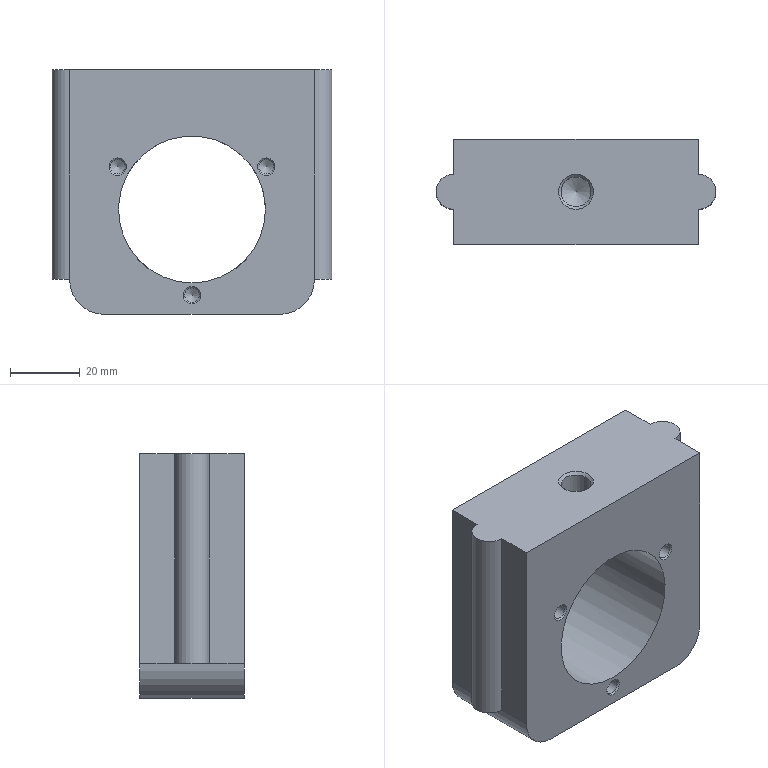Part | STEP file | YBQDJ-YB-3 | 1 solid | 27 faces | box 80 x 30 x 70 mm | volume 107518 mm3 | plane 10 | cylinder 9 | cone 8 | commonest cylinder face diameters 4.2 x3 10 x2 20 x2 8.5 x1 42 x1